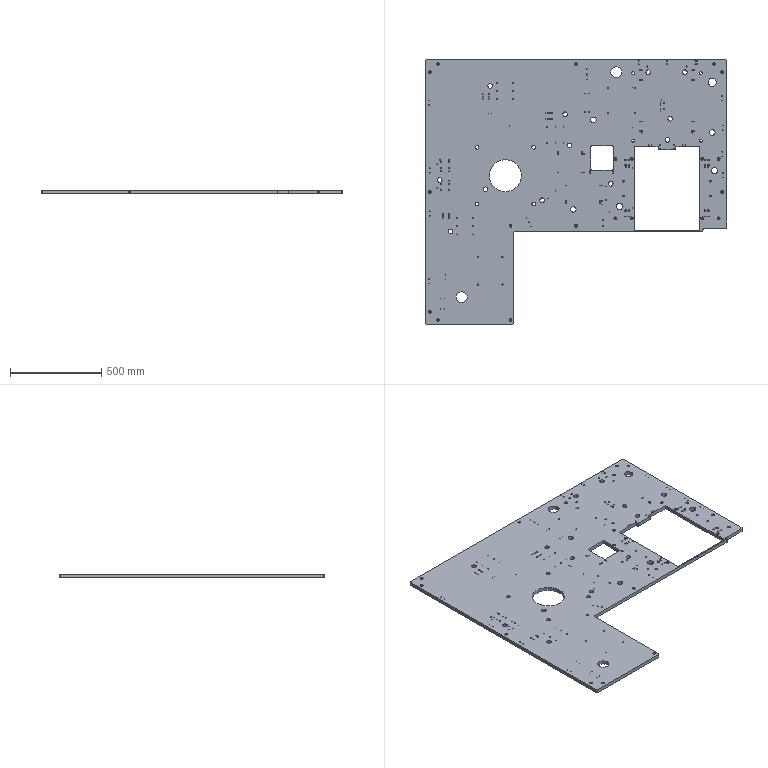Part | STEP file | 11-FG-DB00111 | 1 solid | 716 faces | box 1650 x 1450 x 20 mm | volume 31427316 mm3 | cylinder 573 | cone 96 | plane 47 | commonest cylinder face diameters 4.2 x158 5 x144 3.3 x70 15 x48 9 x40 25 x24